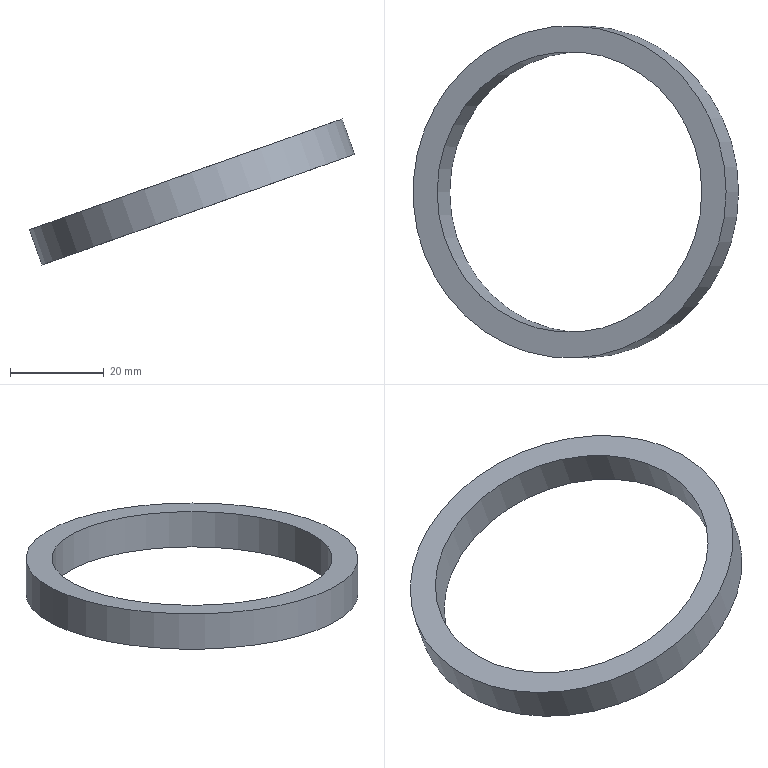Part | STEP file | BRONZE-BUSH1_id526_x_t | 1 solid | 4 faces | box 69.598 x 71 x 31.241 mm | volume 9054 mm3 | plane 2 | cylinder 2 | commonest cylinder face diameters 60 x1 71 x1
STEP:
#1=CARTESIAN_POINT('',(36.868,0.,-70.521));
#2=VERTEX_POINT('',#1);
#3=CARTESIAN_POINT('',(8.589,0.,-80.535));
#4=DIRECTION('',(-0.3338,0.,0.9426));
#5=DIRECTION('',(0.9426,0.,0.3338));
#6=AXIS2_PLACEMENT_3D('',#3,#4,#5);
#7=CIRCLE('',#6,30.);
#8=EDGE_CURVE('',#2,#2,#7,.T.);
#9=ORIENTED_EDGE('',*,*,#8,.T.);
#10=EDGE_LOOP('',(#9));
#11=FACE_BOUND('',#10,.T.);
#12=CARTESIAN_POINT('',(42.053,0.,-68.685));
#13=VERTEX_POINT('',#12);
#14=CARTESIAN_POINT('',(8.589,0.,-80.535));
#15=DIRECTION('',(-0.3338,0.,0.9426));
#16=DIRECTION('',(0.9426,0.,0.3338));
#17=AXIS2_PLACEMENT_3D('',#14,#15,#16);
#18=CIRCLE('',#17,35.5);
#19=EDGE_CURVE('',#13,#13,#18,.T.);
#20=ORIENTED_EDGE('',*,*,#19,.F.);
#21=EDGE_LOOP('',(#20));
#22=FACE_BOUND('',#21,.T.);
#23=CARTESIAN_POINT('',(-47.969,60.,-100.563));
#24=DIRECTION('',(-0.3338,0.,0.9426));
#25=DIRECTION('',(0.9426,0.,0.3338));
#26=AXIS2_PLACEMENT_3D('',#23,#24,#25);
#27=PLANE('',#26);
#28=ADVANCED_FACE('',(#11,#22),#27,.F.);
#29=CARTESIAN_POINT('',(39.382,0.,-61.143));
#30=VERTEX_POINT('',#29);
#31=CARTESIAN_POINT('',(5.919,0.,-72.994));
#32=DIRECTION('',(-0.3338,0.,0.9426));
#33=DIRECTION('',(0.9426,0.,0.3338));
#34=AXIS2_PLACEMENT_3D('',#31,#32,#33);
#35=CIRCLE('',#34,35.5);
#36=EDGE_CURVE('',#30,#30,#35,.T.);
#37=ORIENTED_EDGE('',*,*,#36,.F.);
#38=EDGE_LOOP('',(#37));
#39=FACE_BOUND('',#38,.T.);
#40=ORIENTED_EDGE('',*,*,#19,.T.);
#41=EDGE_LOOP('',(#40));
#42=FACE_BOUND('',#41,.T.);
#43=CARTESIAN_POINT('',(8.589,0.,-80.535));
#44=DIRECTION('',(-0.3338,0.,0.9426));
#45=DIRECTION('',(0.9426,0.,0.3338));
#46=AXIS2_PLACEMENT_3D('',#43,#44,#45);
#47=CYLINDRICAL_SURFACE('',#46,35.5);
#48=ADVANCED_FACE('',(#39,#42),#47,.T.);
#49=CARTESIAN_POINT('',(34.198,0.,-62.979));
#50=VERTEX_POINT('',#49);
#51=CARTESIAN_POINT('',(5.919,0.,-72.994));
#52=DIRECTION('',(0.3338,0.,-0.9426));
#53=DIRECTION('',(0.9426,0.,0.3338));
#54=AXIS2_PLACEMENT_3D('',#51,#52,#53);
#55=CIRCLE('',#54,30.);
#56=EDGE_CURVE('',#50,#50,#55,.T.);
#57=ORIENTED_EDGE('',*,*,#56,.F.);
#58=EDGE_LOOP('',(#57));
#59=FACE_BOUND('',#58,.T.);
#60=ORIENTED_EDGE('',*,*,#8,.F.);
#61=EDGE_LOOP('',(#60));
#62=FACE_BOUND('',#61,.T.);
#63=CARTESIAN_POINT('',(8.589,0.,-80.535));
#64=DIRECTION('',(-0.3338,0.,0.9426));
#65=DIRECTION('',(0.9426,0.,0.3338));
#66=AXIS2_PLACEMENT_3D('',#63,#64,#65);
#67=CYLINDRICAL_SURFACE('',#66,30.);
#68=ADVANCED_FACE('',(#59,#62),#67,.F.);
#69=ORIENTED_EDGE('',*,*,#56,.T.);
#70=EDGE_LOOP('',(#69));
#71=FACE_BOUND('',#70,.T.);
#72=ORIENTED_EDGE('',*,*,#36,.T.);
#73=EDGE_LOOP('',(#72));
#74=FACE_BOUND('',#73,.T.);
#75=CARTESIAN_POINT('',(-50.64,60.,-93.022));
#76=DIRECTION('',(-0.3338,0.,0.9426));
#77=DIRECTION('',(0.9426,0.,0.3338));
#78=AXIS2_PLACEMENT_3D('',#75,#76,#77);
#79=PLANE('',#78);
#80=ADVANCED_FACE('',(#71,#74),#79,.T.);
#81=CLOSED_SHELL('',(#28,#48,#68,#80));
#82=MANIFOLD_SOLID_BREP('',#81);
#83=(LENGTH_UNIT()NAMED_UNIT(*)SI_UNIT(.MILLI.,.METRE.));
#84=UNCERTAINTY_MEASURE_WITH_UNIT(LENGTH_MEASURE(0.00002),#83,'','');
#85=(NAMED_UNIT(*)PLANE_ANGLE_UNIT()SI_UNIT($,.RADIAN.));
#86=PLANE_ANGLE_MEASURE_WITH_UNIT(PLANE_ANGLE_MEASURE(0.01745),#85);
#87=DIMENSIONAL_EXPONENTS(0.,0.,0.,0.,0.,0.,0.);
#88=(CONVERSION_BASED_UNIT('DEGREE',#86)NAMED_UNIT(#87)PLANE_ANGLE_UNIT());
#89=(NAMED_UNIT(*)SI_UNIT($,.STERADIAN.)SOLID_ANGLE_UNIT());
#90=(GEOMETRIC_REPRESENTATION_CONTEXT(3)GLOBAL_UNCERTAINTY_ASSIGNED_CONTEXT((#84))GLOBAL_UNIT_ASSIGNED_CONTEXT((#83,#88,#89))REPRESENTATION_CONTEXT('',''));
#91=ADVANCED_BREP_SHAPE_REPRESENTATION('',(#82),#90);